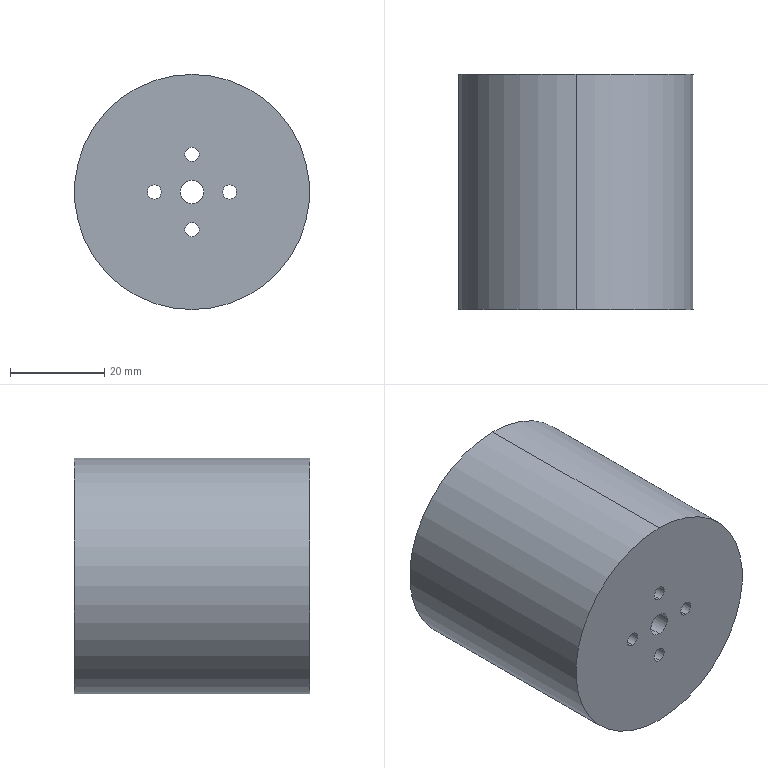Part | STEP file | Dial wheel | 1 solid | 19 faces | box 50 x 50 x 50 mm | volume 41621 mm3 | cylinder 14 | plane 3 | torus 2 | commonest cylinder face diameters 3 x8 5 x2 40 x2 50 x2
STEP:
#1=CARTESIAN_POINT('',(0.,0.,0.));
#2=DIRECTION('',(0.,0.,1.));
#3=DIRECTION('',(1.,0.,0.));
#4=AXIS2_PLACEMENT_3D('',#1,#2,#3);
#5=CARTESIAN_POINT('',(0.,5.,17.));
#6=VERTEX_POINT('',#5);
#7=CARTESIAN_POINT('',(0.,8.,20.));
#8=VERTEX_POINT('',#7);
#9=CARTESIAN_POINT('',(0.,8.,17.));
#10=DIRECTION('',(-1.,0.,0.));
#11=DIRECTION('',(0.,0.,1.));
#12=AXIS2_PLACEMENT_3D('',#9,#10,#11);
#13=CIRCLE('',#12,3.);
#14=CARTESIAN_POINT('',(0.,8.,0.));
#15=DIRECTION('',(0.,1.,0.));
#16=DIRECTION('',(0.,0.,1.));
#17=AXIS2_PLACEMENT_3D('',#14,#15,#16);
#18=TOROIDAL_SURFACE('',#17,17.,3.);
#19=CARTESIAN_POINT('',(6.283,0.));
#20=DIRECTION('',(0.,1.));
#21=VECTOR('',#20,1.);
#22=LINE('',#19,#21);
#23=(GEOMETRIC_REPRESENTATION_CONTEXT(2)PARAMETRIC_REPRESENTATION_CONTEXT()REPRESENTATION_CONTEXT('',''));
#24=DEFINITIONAL_REPRESENTATION('',(#22),#23);
#25=PCURVE('',#18,#24);
#26=CARTESIAN_POINT('',(0.,8.,0.));
#27=DIRECTION('',(0.,1.,0.));
#28=DIRECTION('',(0.,0.,1.));
#29=AXIS2_PLACEMENT_3D('',#26,#27,#28);
#30=TOROIDAL_SURFACE('',#29,17.,3.);
#31=CARTESIAN_POINT('',(0.,0.));
#32=DIRECTION('',(0.,1.));
#33=VECTOR('',#32,1.);
#34=LINE('',#31,#33);
#35=(GEOMETRIC_REPRESENTATION_CONTEXT(2)PARAMETRIC_REPRESENTATION_CONTEXT()REPRESENTATION_CONTEXT('',''));
#36=DEFINITIONAL_REPRESENTATION('',(#34),#35);
#37=PCURVE('',#30,#36);
#38=SURFACE_CURVE('',#13,(#25,#37),.PCURVE_S1.);
#39=EDGE_CURVE('',#6,#8,#38,.T.);
#40=ORIENTED_EDGE('',*,*,#39,.T.);
#41=CARTESIAN_POINT('',(0.,8.,-20.));
#42=VERTEX_POINT('',#41);
#43=CARTESIAN_POINT('',(0.,8.,0.));
#44=DIRECTION('',(0.,-1.,0.));
#45=DIRECTION('',(0.,0.,1.));
#46=AXIS2_PLACEMENT_3D('',#43,#44,#45);
#47=CIRCLE('',#46,20.);
#48=CARTESIAN_POINT('',(6.283,6.283));
#49=DIRECTION('',(-1.,0.));
#50=VECTOR('',#49,1.);
#51=LINE('',#48,#50);
#52=(GEOMETRIC_REPRESENTATION_CONTEXT(2)PARAMETRIC_REPRESENTATION_CONTEXT()REPRESENTATION_CONTEXT('',''));
#53=DEFINITIONAL_REPRESENTATION('',(#51),#52);
#54=PCURVE('',#18,#53);
#55=CARTESIAN_POINT('',(0.,5.,0.));
#56=DIRECTION('',(0.,1.,0.));
#57=DIRECTION('',(0.,0.,1.));
#58=AXIS2_PLACEMENT_3D('',#55,#56,#57);
#59=CYLINDRICAL_SURFACE('',#58,20.);
#60=CARTESIAN_POINT('',(6.283,3.));
#61=DIRECTION('',(-1.,0.));
#62=VECTOR('',#61,1.);
#63=LINE('',#60,#62);
#64=(GEOMETRIC_REPRESENTATION_CONTEXT(2)PARAMETRIC_REPRESENTATION_CONTEXT()REPRESENTATION_CONTEXT('',''));
#65=DEFINITIONAL_REPRESENTATION('',(#63),#64);
#66=PCURVE('',#59,#65);
#67=SURFACE_CURVE('',#47,(#54,#66),.PCURVE_S1.);
#68=EDGE_CURVE('',#8,#42,#67,.T.);
#69=ORIENTED_EDGE('',*,*,#68,.T.);
#70=CARTESIAN_POINT('',(0.,5.,-17.));
#71=VERTEX_POINT('',#70);
#72=CARTESIAN_POINT('',(0.,8.,-17.));
#73=DIRECTION('',(1.,0.,0.));
#74=DIRECTION('',(0.,0.,-1.));
#75=AXIS2_PLACEMENT_3D('',#72,#73,#74);
#76=CIRCLE('',#75,3.);
#77=CARTESIAN_POINT('',(3.142,0.));
#78=DIRECTION('',(0.,1.));
#79=VECTOR('',#78,1.);
#80=LINE('',#77,#79);
#81=(GEOMETRIC_REPRESENTATION_CONTEXT(2)PARAMETRIC_REPRESENTATION_CONTEXT()REPRESENTATION_CONTEXT('',''));
#82=DEFINITIONAL_REPRESENTATION('',(#80),#81);
#83=PCURVE('',#18,#82);
#84=CARTESIAN_POINT('',(3.142,0.));
#85=DIRECTION('',(0.,1.));
#86=VECTOR('',#85,1.);
#87=LINE('',#84,#86);
#88=(GEOMETRIC_REPRESENTATION_CONTEXT(2)PARAMETRIC_REPRESENTATION_CONTEXT()REPRESENTATION_CONTEXT('',''));
#89=DEFINITIONAL_REPRESENTATION('',(#87),#88);
#90=PCURVE('',#30,#89);
#91=SURFACE_CURVE('',#76,(#83,#90),.PCURVE_S1.);
#92=EDGE_CURVE('',#71,#42,#91,.T.);
#93=ORIENTED_EDGE('',*,*,#92,.F.);
#94=CARTESIAN_POINT('',(0.,5.,0.));
#95=DIRECTION('',(0.,1.,0.));
#96=DIRECTION('',(0.,0.,1.));
#97=AXIS2_PLACEMENT_3D('',#94,#95,#96);
#98=CIRCLE('',#97,17.);
#99=CARTESIAN_POINT('',(0.,4.712));
#100=DIRECTION('',(1.,0.));
#101=VECTOR('',#100,1.);
#102=LINE('',#99,#101);
#103=(GEOMETRIC_REPRESENTATION_CONTEXT(2)PARAMETRIC_REPRESENTATION_CONTEXT()REPRESENTATION_CONTEXT('',''));
#104=DEFINITIONAL_REPRESENTATION('',(#102),#103);
#105=PCURVE('',#18,#104);
#106=CARTESIAN_POINT('',(0.,5.,0.));
#107=DIRECTION('',(0.,1.,0.));
#108=DIRECTION('',(0.,0.,1.));
#109=AXIS2_PLACEMENT_3D('',#106,#107,#108);
#110=PLANE('',#109);
#111=CARTESIAN_POINT('',(0.,0.));
#112=DIRECTION('',(1.,0.));
#113=AXIS2_PLACEMENT_2D('',#111,#112);
#114=CIRCLE('',#113,17.);
#115=(GEOMETRIC_REPRESENTATION_CONTEXT(2)PARAMETRIC_REPRESENTATION_CONTEXT()REPRESENTATION_CONTEXT('',''));
#116=DEFINITIONAL_REPRESENTATION('',(#114),#115);
#117=PCURVE('',#110,#116);
#118=SURFACE_CURVE('',#98,(#105,#117),.PCURVE_S1.);
#119=EDGE_CURVE('',#71,#6,#118,.T.);
#120=ORIENTED_EDGE('',*,*,#119,.T.);
#121=EDGE_LOOP('',(#40,#69,#93,#120));
#122=FACE_BOUND('',#121,.F.);
#123=ADVANCED_FACE('',(#122),#18,.F.);
#124=CARTESIAN_POINT('',(0.,50.,20.));
#125=VERTEX_POINT('',#124);
#126=CARTESIAN_POINT('',(0.,5.,20.));
#127=DIRECTION('',(0.,1.,0.));
#128=VECTOR('',#127,1.);
#129=LINE('',#126,#128);
#130=CARTESIAN_POINT('',(6.283,0.));
#131=DIRECTION('',(0.,1.));
#132=VECTOR('',#131,1.);
#133=LINE('',#130,#132);
#134=(GEOMETRIC_REPRESENTATION_CONTEXT(2)PARAMETRIC_REPRESENTATION_CONTEXT()REPRESENTATION_CONTEXT('',''));
#135=DEFINITIONAL_REPRESENTATION('',(#133),#134);
#136=PCURVE('',#59,#135);
#137=CARTESIAN_POINT('',(0.,5.,0.));
#138=DIRECTION('',(0.,1.,0.));
#139=DIRECTION('',(0.,0.,1.));
#140=AXIS2_PLACEMENT_3D('',#137,#138,#139);
#141=CYLINDRICAL_SURFACE('',#140,20.);
#142=CARTESIAN_POINT('',(0.,0.));
#143=DIRECTION('',(0.,1.));
#144=VECTOR('',#143,1.);
#145=LINE('',#142,#144);
#146=(GEOMETRIC_REPRESENTATION_CONTEXT(2)PARAMETRIC_REPRESENTATION_CONTEXT()REPRESENTATION_CONTEXT('',''));
#147=DEFINITIONAL_REPRESENTATION('',(#145),#146);
#148=PCURVE('',#141,#147);
#149=SURFACE_CURVE('',#129,(#136,#148),.PCURVE_S1.);
#150=EDGE_CURVE('',#8,#125,#149,.T.);
#151=ORIENTED_EDGE('',*,*,#150,.T.);
#152=CARTESIAN_POINT('',(0.,50.,-20.));
#153=VERTEX_POINT('',#152);
#154=CARTESIAN_POINT('',(0.,50.,0.));
#155=DIRECTION('',(0.,1.,0.));
#156=DIRECTION('',(0.,0.,1.));
#157=AXIS2_PLACEMENT_3D('',#154,#155,#156);
#158=CIRCLE('',#157,20.);
#159=CARTESIAN_POINT('',(0.,45.));
#160=DIRECTION('',(1.,0.));
#161=VECTOR('',#160,1.);
#162=LINE('',#159,#161);
#163=(GEOMETRIC_REPRESENTATION_CONTEXT(2)PARAMETRIC_REPRESENTATION_CONTEXT()REPRESENTATION_CONTEXT('',''));
#164=DEFINITIONAL_REPRESENTATION('',(#162),#163);
#165=PCURVE('',#59,#164);
#166=CARTESIAN_POINT('',(0.,50.,0.));
#167=DIRECTION('',(0.,1.,0.));
#168=DIRECTION('',(0.,0.,1.));
#169=AXIS2_PLACEMENT_3D('',#166,#167,#168);
#170=PLANE('',#169);
#171=CARTESIAN_POINT('',(0.,0.));
#172=DIRECTION('',(1.,0.));
#173=AXIS2_PLACEMENT_2D('',#171,#172);
#174=CIRCLE('',#173,20.);
#175=(GEOMETRIC_REPRESENTATION_CONTEXT(2)PARAMETRIC_REPRESENTATION_CONTEXT()REPRESENTATION_CONTEXT('',''));
#176=DEFINITIONAL_REPRESENTATION('',(#174),#175);
#177=PCURVE('',#170,#176);
#178=SURFACE_CURVE('',#158,(#165,#177),.PCURVE_S1.);
#179=EDGE_CURVE('',#153,#125,#178,.T.);
#180=ORIENTED_EDGE('',*,*,#179,.F.);
#181=CARTESIAN_POINT('',(0.,5.,-20.));
#182=DIRECTION('',(0.,1.,0.));
#183=VECTOR('',#182,1.);
#184=LINE('',#181,#183);
#185=CARTESIAN_POINT('',(3.142,0.));
#186=DIRECTION('',(0.,1.));
#187=VECTOR('',#186,1.);
#188=LINE('',#185,#187);
#189=(GEOMETRIC_REPRESENTATION_CONTEXT(2)PARAMETRIC_REPRESENTATION_CONTEXT()REPRESENTATION_CONTEXT('',''));
#190=DEFINITIONAL_REPRESENTATION('',(#188),#189);
#191=PCURVE('',#59,#190);
#192=CARTESIAN_POINT('',(3.142,0.));
#193=DIRECTION('',(0.,1.));
#194=VECTOR('',#193,1.);
#195=LINE('',#192,#194);
#196=(GEOMETRIC_REPRESENTATION_CONTEXT(2)PARAMETRIC_REPRESENTATION_CONTEXT()REPRESENTATION_CONTEXT('',''));
#197=DEFINITIONAL_REPRESENTATION('',(#195),#196);
#198=PCURVE('',#141,#197);
#199=SURFACE_CURVE('',#184,(#191,#198),.PCURVE_S1.);
#200=EDGE_CURVE('',#42,#153,#199,.T.);
#201=ORIENTED_EDGE('',*,*,#200,.F.);
#202=ORIENTED_EDGE('',*,*,#68,.F.);
#203=EDGE_LOOP('',(#151,#180,#201,#202));
#204=FACE_BOUND('',#203,.F.);
#205=ADVANCED_FACE('',(#204),#59,.F.);
#206=CARTESIAN_POINT('',(0.,50.,25.));
#207=VERTEX_POINT('',#206);
#208=CARTESIAN_POINT('',(0.,50.,-25.));
#209=VERTEX_POINT('',#208);
#210=CARTESIAN_POINT('',(0.,50.,0.));
#211=DIRECTION('',(0.,1.,0.));
#212=DIRECTION('',(0.,0.,1.));
#213=AXIS2_PLACEMENT_3D('',#210,#211,#212);
#214=CIRCLE('',#213,25.);
#215=CARTESIAN_POINT('',(0.,50.,0.));
#216=DIRECTION('',(0.,-1.,0.));
#217=DIRECTION('',(0.,0.,-1.));
#218=AXIS2_PLACEMENT_3D('',#215,#216,#217);
#219=CYLINDRICAL_SURFACE('',#218,25.);
#220=CARTESIAN_POINT('',(3.142,0.));
#221=DIRECTION('',(-1.,0.));
#222=VECTOR('',#221,1.);
#223=LINE('',#220,#222);
#224=(GEOMETRIC_REPRESENTATION_CONTEXT(2)PARAMETRIC_REPRESENTATION_CONTEXT()REPRESENTATION_CONTEXT('',''));
#225=DEFINITIONAL_REPRESENTATION('',(#223),#224);
#226=PCURVE('',#219,#225);
#227=CARTESIAN_POINT('',(0.,0.));
#228=DIRECTION('',(1.,0.));
#229=AXIS2_PLACEMENT_2D('',#227,#228);
#230=CIRCLE('',#229,25.);
#231=(GEOMETRIC_REPRESENTATION_CONTEXT(2)PARAMETRIC_REPRESENTATION_CONTEXT()REPRESENTATION_CONTEXT('',''));
#232=DEFINITIONAL_REPRESENTATION('',(#230),#231);
#233=PCURVE('',#170,#232);
#234=SURFACE_CURVE('',#214,(#226,#233),.PCURVE_S1.);
#235=EDGE_CURVE('',#207,#209,#234,.T.);
#236=ORIENTED_EDGE('',*,*,#235,.F.);
#237=CARTESIAN_POINT('',(0.,0.,25.));
#238=VERTEX_POINT('',#237);
#239=CARTESIAN_POINT('',(0.,50.,25.));
#240=DIRECTION('',(0.,-1.,0.));
#241=VECTOR('',#240,1.);
#242=LINE('',#239,#241);
#243=CARTESIAN_POINT('',(3.142,0.));
#244=DIRECTION('',(0.,1.));
#245=VECTOR('',#244,1.);
#246=LINE('',#243,#245);
#247=(GEOMETRIC_REPRESENTATION_CONTEXT(2)PARAMETRIC_REPRESENTATION_CONTEXT()REPRESENTATION_CONTEXT('',''));
#248=DEFINITIONAL_REPRESENTATION('',(#246),#247);
#249=PCURVE('',#219,#248);
#250=CARTESIAN_POINT('',(0.,50.,0.));
#251=DIRECTION('',(0.,-1.,0.));
#252=DIRECTION('',(0.,0.,-1.));
#253=AXIS2_PLACEMENT_3D('',#250,#251,#252);
#254=CYLINDRICAL_SURFACE('',#253,25.);
#255=CARTESIAN_POINT('',(3.142,0.));
#256=DIRECTION('',(0.,1.));
#257=VECTOR('',#256,1.);
#258=LINE('',#255,#257);
#259=(GEOMETRIC_REPRESENTATION_CONTEXT(2)PARAMETRIC_REPRESENTATION_CONTEXT()REPRESENTATION_CONTEXT('',''));
#260=DEFINITIONAL_REPRESENTATION('',(#258),#259);
#261=PCURVE('',#254,#260);
#262=SURFACE_CURVE('',#242,(#249,#261),.PCURVE_S1.);
#263=EDGE_CURVE('',#207,#238,#262,.T.);
#264=ORIENTED_EDGE('',*,*,#263,.T.);
#265=CARTESIAN_POINT('',(0.,0.,-25.));
#266=VERTEX_POINT('',#265);
#267=CARTESIAN_POINT('',(0.,0.,0.));
#268=DIRECTION('',(0.,1.,0.));
#269=DIRECTION('',(0.,0.,1.));
#270=AXIS2_PLACEMENT_3D('',#267,#268,#269);
#271=CIRCLE('',#270,25.);
#272=CARTESIAN_POINT('',(3.142,50.));
#273=DIRECTION('',(-1.,0.));
#274=VECTOR('',#273,1.);
#275=LINE('',#272,#274);
#276=(GEOMETRIC_REPRESENTATION_CONTEXT(2)PARAMETRIC_REPRESENTATION_CONTEXT()REPRESENTATION_CONTEXT('',''));
#277=DEFINITIONAL_REPRESENTATION('',(#275),#276);
#278=PCURVE('',#219,#277);
#279=CARTESIAN_POINT('',(0.,0.,0.));
#280=DIRECTION('',(0.,1.,0.));
#281=DIRECTION('',(0.,0.,1.));
#282=AXIS2_PLACEMENT_3D('',#279,#280,#281);
#283=PLANE('',#282);
#284=CARTESIAN_POINT('',(0.,0.));
#285=DIRECTION('',(1.,0.));
#286=AXIS2_PLACEMENT_2D('',#284,#285);
#287=CIRCLE('',#286,25.);
#288=(GEOMETRIC_REPRESENTATION_CONTEXT(2)PARAMETRIC_REPRESENTATION_CONTEXT()REPRESENTATION_CONTEXT('',''));
#289=DEFINITIONAL_REPRESENTATION('',(#287),#288);
#290=PCURVE('',#283,#289);
#291=SURFACE_CURVE('',#271,(#278,#290),.PCURVE_S1.);
#292=EDGE_CURVE('',#238,#266,#291,.T.);
#293=ORIENTED_EDGE('',*,*,#292,.T.);
#294=CARTESIAN_POINT('',(0.,50.,-25.));
#295=DIRECTION('',(0.,-1.,0.));
#296=VECTOR('',#295,1.);
#297=LINE('',#294,#296);
#298=CARTESIAN_POINT('',(0.,0.));
#299=DIRECTION('',(0.,1.));
#300=VECTOR('',#299,1.);
#301=LINE('',#298,#300);
#302=(GEOMETRIC_REPRESENTATION_CONTEXT(2)PARAMETRIC_REPRESENTATION_CONTEXT()REPRESENTATION_CONTEXT('',''));
#303=DEFINITIONAL_REPRESENTATION('',(#301),#302);
#304=PCURVE('',#219,#303);
#305=CARTESIAN_POINT('',(6.283,0.));
#306=DIRECTION('',(0.,1.));
#307=VECTOR('',#306,1.);
#308=LINE('',#305,#307);
#309=(GEOMETRIC_REPRESENTATION_CONTEXT(2)PARAMETRIC_REPRESENTATION_CONTEXT()REPRESENTATION_CONTEXT('',''));
#310=DEFINITIONAL_REPRESENTATION('',(#308),#309);
#311=PCURVE('',#254,#310);
#312=SURFACE_CURVE('',#297,(#304,#311),.PCURVE_S1.);
#313=EDGE_CURVE('',#209,#266,#312,.T.);
#314=ORIENTED_EDGE('',*,*,#313,.F.);
#315=EDGE_LOOP('',(#236,#264,#293,#314));
#316=FACE_BOUND('',#315,.T.);
#317=ADVANCED_FACE('',(#316),#219,.T.);
#318=CARTESIAN_POINT('',(0.,5.,6.5));
#319=VERTEX_POINT('',#318);
#320=CARTESIAN_POINT('',(0.,0.,6.5));
#321=VERTEX_POINT('',#320);
#322=CARTESIAN_POINT('',(0.,128.,6.5));
#323=DIRECTION('',(0.,-1.,0.));
#324=VECTOR('',#323,1.);
#325=LINE('',#322,#324);
#326=CARTESIAN_POINT('',(0.,128.,8.));
#327=DIRECTION('',(0.,-1.,0.));
#328=DIRECTION('',(0.,0.,-1.));
#329=AXIS2_PLACEMENT_3D('',#326,#327,#328);
#330=CYLINDRICAL_SURFACE('',#329,1.5);
#331=CARTESIAN_POINT('',(6.283,0.));
#332=DIRECTION('',(0.,1.));
#333=VECTOR('',#332,1.);
#334=LINE('',#331,#333);
#335=(GEOMETRIC_REPRESENTATION_CONTEXT(2)PARAMETRIC_REPRESENTATION_CONTEXT()REPRESENTATION_CONTEXT('',''));
#336=DEFINITIONAL_REPRESENTATION('',(#334),#335);
#337=PCURVE('',#330,#336);
#338=CARTESIAN_POINT('',(0.,128.,8.));
#339=DIRECTION('',(0.,-1.,0.));
#340=DIRECTION('',(0.,0.,-1.));
#341=AXIS2_PLACEMENT_3D('',#338,#339,#340);
#342=CYLINDRICAL_SURFACE('',#341,1.5);
#343=CARTESIAN_POINT('',(0.,0.));
#344=DIRECTION('',(0.,1.));
#345=VECTOR('',#344,1.);
#346=LINE('',#343,#345);
#347=(GEOMETRIC_REPRESENTATION_CONTEXT(2)PARAMETRIC_REPRESENTATION_CONTEXT()REPRESENTATION_CONTEXT('',''));
#348=DEFINITIONAL_REPRESENTATION('',(#346),#347);
#349=PCURVE('',#342,#348);
#350=SURFACE_CURVE('',#325,(#337,#349),.PCURVE_S1.);
#351=EDGE_CURVE('',#319,#321,#350,.T.);
#352=ORIENTED_EDGE('',*,*,#351,.T.);
#353=CARTESIAN_POINT('',(0.,0.,9.5));
#354=VERTEX_POINT('',#353);
#355=CARTESIAN_POINT('',(0.,0.,8.));
#356=DIRECTION('',(0.,1.,0.));
#357=DIRECTION('',(0.,0.,1.));
#358=AXIS2_PLACEMENT_3D('',#355,#356,#357);
#359=CIRCLE('',#358,1.5);
#360=CARTESIAN_POINT('',(9.425,128.));
#361=DIRECTION('',(-1.,0.));
#362=VECTOR('',#361,1.);
#363=LINE('',#360,#362);
#364=(GEOMETRIC_REPRESENTATION_CONTEXT(2)PARAMETRIC_REPRESENTATION_CONTEXT()REPRESENTATION_CONTEXT('',''));
#365=DEFINITIONAL_REPRESENTATION('',(#363),#364);
#366=PCURVE('',#330,#365);
#367=CARTESIAN_POINT('',(8.,0.));
#368=DIRECTION('',(1.,0.));
#369=AXIS2_PLACEMENT_2D('',#367,#368);
#370=CIRCLE('',#369,1.5);
#371=(GEOMETRIC_REPRESENTATION_CONTEXT(2)PARAMETRIC_REPRESENTATION_CONTEXT()REPRESENTATION_CONTEXT('',''));
#372=DEFINITIONAL_REPRESENTATION('',(#370),#371);
#373=PCURVE('',#283,#372);
#374=SURFACE_CURVE('',#359,(#366,#373),.PCURVE_S1.);
#375=EDGE_CURVE('',#321,#354,#374,.T.);
#376=ORIENTED_EDGE('',*,*,#375,.T.);
#377=CARTESIAN_POINT('',(0.,5.,9.5));
#378=VERTEX_POINT('',#377);
#379=CARTESIAN_POINT('',(0.,128.,9.5));
#380=DIRECTION('',(0.,-1.,0.));
#381=VECTOR('',#380,1.);
#382=LINE('',#379,#381);
#383=CARTESIAN_POINT('',(3.142,0.));
#384=DIRECTION('',(0.,1.));
#385=VECTOR('',#384,1.);
#386=LINE('',#383,#385);
#387=(GEOMETRIC_REPRESENTATION_CONTEXT(2)PARAMETRIC_REPRESENTATION_CONTEXT()REPRESENTATION_CONTEXT('',''));
#388=DEFINITIONAL_REPRESENTATION('',(#386),#387);
#389=PCURVE('',#330,#388);
#390=CARTESIAN_POINT('',(3.142,0.));
#391=DIRECTION('',(0.,1.));
#392=VECTOR('',#391,1.);
#393=LINE('',#390,#392);
#394=(GEOMETRIC_REPRESENTATION_CONTEXT(2)PARAMETRIC_REPRESENTATION_CONTEXT()REPRESENTATION_CONTEXT('',''));
#395=DEFINITIONAL_REPRESENTATION('',(#393),#394);
#396=PCURVE('',#342,#395);
#397=SURFACE_CURVE('',#382,(#389,#396),.PCURVE_S1.);
#398=EDGE_CURVE('',#378,#354,#397,.T.);
#399=ORIENTED_EDGE('',*,*,#398,.F.);
#400=CARTESIAN_POINT('',(0.,5.,8.));
#401=DIRECTION('',(0.,-1.,0.));
#402=DIRECTION('',(0.,0.,1.));
#403=AXIS2_PLACEMENT_3D('',#400,#401,#402);
#404=CIRCLE('',#403,1.5);
#405=CARTESIAN_POINT('',(3.142,123.));
#406=DIRECTION('',(1.,0.));
#407=VECTOR('',#406,1.);
#408=LINE('',#405,#407);
#409=(GEOMETRIC_REPRESENTATION_CONTEXT(2)PARAMETRIC_REPRESENTATION_CONTEXT()REPRESENTATION_CONTEXT('',''));
#410=DEFINITIONAL_REPRESENTATION('',(#408),#409);
#411=PCURVE('',#330,#410);
#412=CARTESIAN_POINT('',(9.5,0.));
#413=CARTESIAN_POINT('',(9.5,-2.598));
#414=CARTESIAN_POINT('',(7.25,-1.299));
#415=CARTESIAN_POINT('',(5.,0.));
#416=CARTESIAN_POINT('',(7.25,1.299));
#417=CARTESIAN_POINT('',(9.5,2.598));
#418=CARTESIAN_POINT('',(9.5,0.));
#419=(BOUNDED_CURVE()B_SPLINE_CURVE(2,(#412,#413,#414,#415,#416,#417,#418),.UNSPECIFIED.,.T.,.F.)B_SPLINE_CURVE_WITH_KNOTS((1,2,2,2,2,1),(-2.094,0.,2.094,4.189,6.283,8.378),.UNSPECIFIED.)CURVE()GEOMETRIC_REPRESENTATION_ITEM()RATIONAL_B_SPLINE_CURVE((1.,0.5,1.,0.5,1.,0.5,1.))REPRESENTATION_ITEM(''));
#420=(GEOMETRIC_REPRESENTATION_CONTEXT(2)PARAMETRIC_REPRESENTATION_CONTEXT()REPRESENTATION_CONTEXT('',''));
#421=DEFINITIONAL_REPRESENTATION('',(#419),#420);
#422=PCURVE('',#110,#421);
#423=SURFACE_CURVE('',#404,(#411,#422),.PCURVE_S1.);
#424=EDGE_CURVE('',#378,#319,#423,.T.);
#425=ORIENTED_EDGE('',*,*,#424,.T.);
#426=EDGE_LOOP('',(#352,#376,#399,#425));
#427=FACE_BOUND('',#426,.F.);
#428=ADVANCED_FACE('',(#427),#330,.F.);
#429=CARTESIAN_POINT('',(0.,5.,-9.5));
#430=VERTEX_POINT('',#429);
#431=CARTESIAN_POINT('',(0.,0.,-9.5));
#432=VERTEX_POINT('',#431);
#433=CARTESIAN_POINT('',(0.,128.,-9.5));
#434=DIRECTION('',(0.,-1.,0.));
#435=VECTOR('',#434,1.);
#436=LINE('',#433,#435);
#437=CARTESIAN_POINT('',(0.,128.,-8.));
#438=DIRECTION('',(0.,-1.,0.));
#439=DIRECTION('',(0.,0.,-1.));
#440=AXIS2_PLACEMENT_3D('',#437,#438,#439);
#441=CYLINDRICAL_SURFACE('',#440,1.5);
#442=CARTESIAN_POINT('',(6.283,0.));
#443=DIRECTION('',(0.,1.));
#444=VECTOR('',#443,1.);
#445=LINE('',#442,#444);
#446=(GEOMETRIC_REPRESENTATION_CONTEXT(2)PARAMETRIC_REPRESENTATION_CONTEXT()REPRESENTATION_CONTEXT('',''));
#447=DEFINITIONAL_REPRESENTATION('',(#445),#446);
#448=PCURVE('',#441,#447);
#449=CARTESIAN_POINT('',(0.,128.,-8.));
#450=DIRECTION('',(0.,-1.,0.));
#451=DIRECTION('',(0.,0.,-1.));
#452=AXIS2_PLACEMENT_3D('',#449,#450,#451);
#453=CYLINDRICAL_SURFACE('',#452,1.5);
#454=CARTESIAN_POINT('',(0.,0.));
#455=DIRECTION('',(0.,1.));
#456=VECTOR('',#455,1.);
#457=LINE('',#454,#456);
#458=(GEOMETRIC_REPRESENTATION_CONTEXT(2)PARAMETRIC_REPRESENTATION_CONTEXT()REPRESENTATION_CONTEXT('',''));
#459=DEFINITIONAL_REPRESENTATION('',(#457),#458);
#460=PCURVE('',#453,#459);
#461=SURFACE_CURVE('',#436,(#448,#460),.PCURVE_S1.);
#462=EDGE_CURVE('',#430,#432,#461,.T.);
#463=ORIENTED_EDGE('',*,*,#462,.T.);
#464=CARTESIAN_POINT('',(0.,0.,-6.5));
#465=VERTEX_POINT('',#464);
#466=CARTESIAN_POINT('',(0.,0.,-8.));
#467=DIRECTION('',(0.,1.,0.));
#468=DIRECTION('',(0.,0.,1.));
#469=AXIS2_PLACEMENT_3D('',#466,#467,#468);
#470=CIRCLE('',#469,1.5);
#471=CARTESIAN_POINT('',(9.425,128.));
#472=DIRECTION('',(-1.,0.));
#473=VECTOR('',#472,1.);
#474=LINE('',#471,#473);
#475=(GEOMETRIC_REPRESENTATION_CONTEXT(2)PARAMETRIC_REPRESENTATION_CONTEXT()REPRESENTATION_CONTEXT('',''));
#476=DEFINITIONAL_REPRESENTATION('',(#474),#475);
#477=PCURVE('',#441,#476);
#478=CARTESIAN_POINT('',(-8.,0.));
#479=DIRECTION('',(1.,0.));
#480=AXIS2_PLACEMENT_2D('',#478,#479);
#481=CIRCLE('',#480,1.5);
#482=(GEOMETRIC_REPRESENTATION_CONTEXT(2)PARAMETRIC_REPRESENTATION_CONTEXT()REPRESENTATION_CONTEXT('',''));
#483=DEFINITIONAL_REPRESENTATION('',(#481),#482);
#484=PCURVE('',#283,#483);
#485=SURFACE_CURVE('',#470,(#477,#484),.PCURVE_S1.);
#486=EDGE_CURVE('',#432,#465,#485,.T.);
#487=ORIENTED_EDGE('',*,*,#486,.T.);
#488=CARTESIAN_POINT('',(0.,5.,-6.5));
#489=VERTEX_POINT('',#488);
#490=CARTESIAN_POINT('',(0.,128.,-6.5));
#491=DIRECTION('',(0.,-1.,0.));
#492=VECTOR('',#491,1.);
#493=LINE('',#490,#492);
#494=CARTESIAN_POINT('',(3.142,0.));
#495=DIRECTION('',(0.,1.));
#496=VECTOR('',#495,1.);
#497=LINE('',#494,#496);
#498=(GEOMETRIC_REPRESENTATION_CONTEXT(2)PARAMETRIC_REPRESENTATION_CONTEXT()REPRESENTATION_CONTEXT('',''));
#499=DEFINITIONAL_REPRESENTATION('',(#497),#498);
#500=PCURVE('',#441,#499);
#501=CARTESIAN_POINT('',(3.142,0.));
#502=DIRECTION('',(0.,1.));
#503=VECTOR('',#502,1.);
#504=LINE('',#501,#503);
#505=(GEOMETRIC_REPRESENTATION_CONTEXT(2)PARAMETRIC_REPRESENTATION_CONTEXT()REPRESENTATION_CONTEXT('',''));
#506=DEFINITIONAL_REPRESENTATION('',(#504),#505);
#507=PCURVE('',#453,#506);
#508=SURFACE_CURVE('',#493,(#500,#507),.PCURVE_S1.);
#509=EDGE_CURVE('',#489,#465,#508,.T.);
#510=ORIENTED_EDGE('',*,*,#509,.F.);
#511=CARTESIAN_POINT('',(0.,5.,-8.));
#512=DIRECTION('',(0.,-1.,0.));
#513=DIRECTION('',(0.,0.,1.));
#514=AXIS2_PLACEMENT_3D('',#511,#512,#513);
#515=CIRCLE('',#514,1.5);
#516=CARTESIAN_POINT('',(3.142,123.));
#517=DIRECTION('',(1.,0.));
#518=VECTOR('',#517,1.);
#519=LINE('',#516,#518);
#520=(GEOMETRIC_REPRESENTATION_CONTEXT(2)PARAMETRIC_REPRESENTATION_CONTEXT()REPRESENTATION_CONTEXT('',''));
#521=DEFINITIONAL_REPRESENTATION('',(#519),#520);
#522=PCURVE('',#441,#521);
#523=CARTESIAN_POINT('',(-6.5,0.));
#524=CARTESIAN_POINT('',(-6.5,-2.598));
#525=CARTESIAN_POINT('',(-8.75,-1.299));
#526=CARTESIAN_POINT('',(-11.,0.));
#527=CARTESIAN_POINT('',(-8.75,1.299));
#528=CARTESIAN_POINT('',(-6.5,2.598));
#529=CARTESIAN_POINT('',(-6.5,0.));
#530=(BOUNDED_CURVE()B_SPLINE_CURVE(2,(#523,#524,#525,#526,#527,#528,#529),.UNSPECIFIED.,.T.,.F.)B_SPLINE_CURVE_WITH_KNOTS((1,2,2,2,2,1),(-2.094,0.,2.094,4.189,6.283,8.378),.UNSPECIFIED.)CURVE()GEOMETRIC_REPRESENTATION_ITEM()RATIONAL_B_SPLINE_CURVE((1.,0.5,1.,0.5,1.,0.5,1.))REPRESENTATION_ITEM(''));
#531=(GEOMETRIC_REPRESENTATION_CONTEXT(2)PARAMETRIC_REPRESENTATION_CONTEXT()REPRESENTATION_CONTEXT('',''));
#532=DEFINITIONAL_REPRESENTATION('',(#530),#531);
#533=PCURVE('',#110,#532);
#534=SURFACE_CURVE('',#515,(#522,#533),.PCURVE_S1.);
#535=EDGE_CURVE('',#489,#430,#534,.T.);
#536=ORIENTED_EDGE('',*,*,#535,.T.);
#537=EDGE_LOOP('',(#463,#487,#510,#536));
#538=FACE_BOUND('',#537,.F.);
#539=ADVANCED_FACE('',(#538),#441,.F.);
#540=CARTESIAN_POINT('',(-8.,5.,-1.5));
#541=VERTEX_POINT('',#540);
#542=CARTESIAN_POINT('',(-8.,0.,-1.5));
#543=VERTEX_POINT('',#542);
#544=CARTESIAN_POINT('',(-8.,128.,-1.5));
#545=DIRECTION('',(0.,-1.,0.));
#546=VECTOR('',#545,1.);
#547=LINE('',#544,#546);
#548=CARTESIAN_POINT('',(-8.,128.,0.));
#549=DIRECTION('',(0.,-1.,0.));
#550=DIRECTION('',(0.,0.,-1.));
#551=AXIS2_PLACEMENT_3D('',#548,#549,#550);
#552=CYLINDRICAL_SURFACE('',#551,1.5);
#553=CARTESIAN_POINT('',(6.283,0.));
#554=DIRECTION('',(0.,1.));
#555=VECTOR('',#554,1.);
#556=LINE('',#553,#555);
#557=(GEOMETRIC_REPRESENTATION_CONTEXT(2)PARAMETRIC_REPRESENTATION_CONTEXT()REPRESENTATION_CONTEXT('',''));
#558=DEFINITIONAL_REPRESENTATION('',(#556),#557);
#559=PCURVE('',#552,#558);
#560=CARTESIAN_POINT('',(-8.,128.,0.));
#561=DIRECTION('',(0.,-1.,0.));
#562=DIRECTION('',(0.,0.,-1.));
#563=AXIS2_PLACEMENT_3D('',#560,#561,#562);
#564=CYLINDRICAL_SURFACE('',#563,1.5);
#565=CARTESIAN_POINT('',(0.,0.));
#566=DIRECTION('',(0.,1.));
#567=VECTOR('',#566,1.);
#568=LINE('',#565,#567);
#569=(GEOMETRIC_REPRESENTATION_CONTEXT(2)PARAMETRIC_REPRESENTATION_CONTEXT()REPRESENTATION_CONTEXT('',''));
#570=DEFINITIONAL_REPRESENTATION('',(#568),#569);
#571=PCURVE('',#564,#570);
#572=SURFACE_CURVE('',#547,(#559,#571),.PCURVE_S1.);
#573=EDGE_CURVE('',#541,#543,#572,.T.);
#574=ORIENTED_EDGE('',*,*,#573,.T.);
#575=CARTESIAN_POINT('',(-8.,0.,1.5));
#576=VERTEX_POINT('',#575);
#577=CARTESIAN_POINT('',(-8.,0.,0.));
#578=DIRECTION('',(0.,1.,0.));
#579=DIRECTION('',(0.,0.,1.));
#580=AXIS2_PLACEMENT_3D('',#577,#578,#579);
#581=CIRCLE('',#580,1.5);
#582=CARTESIAN_POINT('',(9.425,128.));
#583=DIRECTION('',(-1.,0.));
#584=VECTOR('',#583,1.);
#585=LINE('',#582,#584);
#586=(GEOMETRIC_REPRESENTATION_CONTEXT(2)PARAMETRIC_REPRESENTATION_CONTEXT()REPRESENTATION_CONTEXT('',''));
#587=DEFINITIONAL_REPRESENTATION('',(#585),#586);
#588=PCURVE('',#552,#587);
#589=CARTESIAN_POINT('',(0.,-8.));
#590=DIRECTION('',(1.,0.));
#591=AXIS2_PLACEMENT_2D('',#589,#590);
#592=CIRCLE('',#591,1.5);
#593=(GEOMETRIC_REPRESENTATION_CONTEXT(2)PARAMETRIC_REPRESENTATION_CONTEXT()REPRESENTATION_CONTEXT('',''));
#594=DEFINITIONAL_REPRESENTATION('',(#592),#593);
#595=PCURVE('',#283,#594);
#596=SURFACE_CURVE('',#581,(#588,#595),.PCURVE_S1.);
#597=EDGE_CURVE('',#543,#576,#596,.T.);
#598=ORIENTED_EDGE('',*,*,#597,.T.);
#599=CARTESIAN_POINT('',(-8.,5.,1.5));
#600=VERTEX_POINT('',#599);
#601=CARTESIAN_POINT('',(-8.,128.,1.5));
#602=DIRECTION('',(0.,-1.,0.));
#603=VECTOR('',#602,1.);
#604=LINE('',#601,#603);
#605=CARTESIAN_POINT('',(3.142,0.));
#606=DIRECTION('',(0.,1.));
#607=VECTOR('',#606,1.);
#608=LINE('',#605,#607);
#609=(GEOMETRIC_REPRESENTATION_CONTEXT(2)PARAMETRIC_REPRESENTATION_CONTEXT()REPRESENTATION_CONTEXT('',''));
#610=DEFINITIONAL_REPRESENTATION('',(#608),#609);
#611=PCURVE('',#552,#610);
#612=CARTESIAN_POINT('',(3.142,0.));
#613=DIRECTION('',(0.,1.));
#614=VECTOR('',#613,1.);
#615=LINE('',#612,#614);
#616=(GEOMETRIC_REPRESENTATION_CONTEXT(2)PARAMETRIC_REPRESENTATION_CONTEXT()REPRESENTATION_CONTEXT('',''));
#617=DEFINITIONAL_REPRESENTATION('',(#615),#616);
#618=PCURVE('',#564,#617);
#619=SURFACE_CURVE('',#604,(#611,#618),.PCURVE_S1.);
#620=EDGE_CURVE('',#600,#576,#619,.T.);
#621=ORIENTED_EDGE('',*,*,#620,.F.);
#622=CARTESIAN_POINT('',(-8.,5.,0.));
#623=DIRECTION('',(0.,-1.,0.));
#624=DIRECTION('',(0.,0.,1.));
#625=AXIS2_PLACEMENT_3D('',#622,#623,#624);
#626=CIRCLE('',#625,1.5);
#627=CARTESIAN_POINT('',(3.142,123.));
#628=DIRECTION('',(1.,0.));
#629=VECTOR('',#628,1.);
#630=LINE('',#627,#629);
#631=(GEOMETRIC_REPRESENTATION_CONTEXT(2)PARAMETRIC_REPRESENTATION_CONTEXT()REPRESENTATION_CONTEXT('',''));
#632=DEFINITIONAL_REPRESENTATION('',(#630),#631);
#633=PCURVE('',#552,#632);
#634=CARTESIAN_POINT('',(1.5,-8.));
#635=CARTESIAN_POINT('',(1.5,-10.598));
#636=CARTESIAN_POINT('',(-0.75,-9.299));
#637=CARTESIAN_POINT('',(-3.,-8.));
#638=CARTESIAN_POINT('',(-0.75,-6.701));
#639=CARTESIAN_POINT('',(1.5,-5.402));
#640=CARTESIAN_POINT('',(1.5,-8.));
#641=(BOUNDED_CURVE()B_SPLINE_CURVE(2,(#634,#635,#636,#637,#638,#639,#640),.UNSPECIFIED.,.T.,.F.)B_SPLINE_CURVE_WITH_KNOTS((1,2,2,2,2,1),(-2.094,0.,2.094,4.189,6.283,8.378),.UNSPECIFIED.)CURVE()GEOMETRIC_REPRESENTATION_ITEM()RATIONAL_B_SPLINE_CURVE((1.,0.5,1.,0.5,1.,0.5,1.))REPRESENTATION_ITEM(''));
#642=(GEOMETRIC_REPRESENTATION_CONTEXT(2)PARAMETRIC_REPRESENTATION_CONTEXT()REPRESENTATION_CONTEXT('',''));
#643=DEFINITIONAL_REPRESENTATION('',(#641),#642);
#644=PCURVE('',#110,#643);
#645=SURFACE_CURVE('',#626,(#633,#644),.PCURVE_S1.);
#646=EDGE_CURVE('',#600,#541,#645,.T.);
#647=ORIENTED_EDGE('',*,*,#646,.T.);
#648=EDGE_LOOP('',(#574,#598,#621,#647));
#649=FACE_BOUND('',#648,.F.);
#650=ADVANCED_FACE('',(#649),#552,.F.);
#651=CARTESIAN_POINT('',(8.,5.,-1.5));
#652=VERTEX_POINT('',#651);
#653=CARTESIAN_POINT('',(8.,0.,-1.5));
#654=VERTEX_POINT('',#653);
#655=CARTESIAN_POINT('',(8.,128.,-1.5));
#656=DIRECTION('',(0.,-1.,0.));
#657=VECTOR('',#656,1.);
#658=LINE('',#655,#657);
#659=CARTESIAN_POINT('',(8.,128.,0.));
#660=DIRECTION('',(0.,-1.,0.));
#661=DIRECTION('',(0.,0.,-1.));
#662=AXIS2_PLACEMENT_3D('',#659,#660,#661);
#663=CYLINDRICAL_SURFACE('',#662,1.5);
#664=CARTESIAN_POINT('',(6.283,0.));
#665=DIRECTION('',(0.,1.));
#666=VECTOR('',#665,1.);
#667=LINE('',#664,#666);
#668=(GEOMETRIC_REPRESENTATION_CONTEXT(2)PARAMETRIC_REPRESENTATION_CONTEXT()REPRESENTATION_CONTEXT('',''));
#669=DEFINITIONAL_REPRESENTATION('',(#667),#668);
#670=PCURVE('',#663,#669);
#671=CARTESIAN_POINT('',(8.,128.,0.));
#672=DIRECTION('',(0.,-1.,0.));
#673=DIRECTION('',(0.,0.,-1.));
#674=AXIS2_PLACEMENT_3D('',#671,#672,#673);
#675=CYLINDRICAL_SURFACE('',#674,1.5);
#676=CARTESIAN_POINT('',(0.,0.));
#677=DIRECTION('',(0.,1.));
#678=VECTOR('',#677,1.);
#679=LINE('',#676,#678);
#680=(GEOMETRIC_REPRESENTATION_CONTEXT(2)PARAMETRIC_REPRESENTATION_CONTEXT()REPRESENTATION_CONTEXT('',''));
#681=DEFINITIONAL_REPRESENTATION('',(#679),#680);
#682=PCURVE('',#675,#681);
#683=SURFACE_CURVE('',#658,(#670,#682),.PCURVE_S1.);
#684=EDGE_CURVE('',#652,#654,#683,.T.);
#685=ORIENTED_EDGE('',*,*,#684,.T.);
#686=CARTESIAN_POINT('',(8.,0.,1.5));
#687=VERTEX_POINT('',#686);
#688=CARTESIAN_POINT('',(8.,0.,0.));
#689=DIRECTION('',(0.,1.,0.));
#690=DIRECTION('',(0.,0.,1.));
#691=AXIS2_PLACEMENT_3D('',#688,#689,#690);
#692=CIRCLE('',#691,1.5);
#693=CARTESIAN_POINT('',(9.425,128.));
#694=DIRECTION('',(-1.,0.));
#695=VECTOR('',#694,1.);
#696=LINE('',#693,#695);
#697=(GEOMETRIC_REPRESENTATION_CONTEXT(2)PARAMETRIC_REPRESENTATION_CONTEXT()REPRESENTATION_CONTEXT('',''));
#698=DEFINITIONAL_REPRESENTATION('',(#696),#697);
#699=PCURVE('',#663,#698);
#700=CARTESIAN_POINT('',(0.,8.));
#701=DIRECTION('',(1.,0.));
#702=AXIS2_PLACEMENT_2D('',#700,#701);
#703=CIRCLE('',#702,1.5);
#704=(GEOMETRIC_REPRESENTATION_CONTEXT(2)PARAMETRIC_REPRESENTATION_CONTEXT()REPRESENTATION_CONTEXT('',''));
#705=DEFINITIONAL_REPRESENTATION('',(#703),#704);
#706=PCURVE('',#283,#705);
#707=SURFACE_CURVE('',#692,(#699,#706),.PCURVE_S1.);
#708=EDGE_CURVE('',#654,#687,#707,.T.);
#709=ORIENTED_EDGE('',*,*,#708,.T.);
#710=CARTESIAN_POINT('',(8.,5.,1.5));
#711=VERTEX_POINT('',#710);
#712=CARTESIAN_POINT('',(8.,128.,1.5));
#713=DIRECTION('',(0.,-1.,0.));
#714=VECTOR('',#713,1.);
#715=LINE('',#712,#714);
#716=CARTESIAN_POINT('',(3.142,0.));
#717=DIRECTION('',(0.,1.));
#718=VECTOR('',#717,1.);
#719=LINE('',#716,#718);
#720=(GEOMETRIC_REPRESENTATION_CONTEXT(2)PARAMETRIC_REPRESENTATION_CONTEXT()REPRESENTATION_CONTEXT('',''));
#721=DEFINITIONAL_REPRESENTATION('',(#719),#720);
#722=PCURVE('',#663,#721);
#723=CARTESIAN_POINT('',(3.142,0.));
#724=DIRECTION('',(0.,1.));
#725=VECTOR('',#724,1.);
#726=LINE('',#723,#725);
#727=(GEOMETRIC_REPRESENTATION_CONTEXT(2)PARAMETRIC_REPRESENTATION_CONTEXT()REPRESENTATION_CONTEXT('',''));
#728=DEFINITIONAL_REPRESENTATION('',(#726),#727);
#729=PCURVE('',#675,#728);
#730=SURFACE_CURVE('',#715,(#722,#729),.PCURVE_S1.);
#731=EDGE_CURVE('',#711,#687,#730,.T.);
#732=ORIENTED_EDGE('',*,*,#731,.F.);
#733=CARTESIAN_POINT('',(8.,5.,0.));
#734=DIRECTION('',(0.,-1.,0.));
#735=DIRECTION('',(0.,0.,1.));
#736=AXIS2_PLACEMENT_3D('',#733,#734,#735);
#737=CIRCLE('',#736,1.5);
#738=CARTESIAN_POINT('',(3.142,123.));
#739=DIRECTION('',(1.,0.));
#740=VECTOR('',#739,1.);
#741=LINE('',#738,#740);
#742=(GEOMETRIC_REPRESENTATION_CONTEXT(2)PARAMETRIC_REPRESENTATION_CONTEXT()REPRESENTATION_CONTEXT('',''));
#743=DEFINITIONAL_REPRESENTATION('',(#741),#742);
#744=PCURVE('',#663,#743);
#745=CARTESIAN_POINT('',(1.5,8.));
#746=CARTESIAN_POINT('',(1.5,5.402));
#747=CARTESIAN_POINT('',(-0.75,6.701));
#748=CARTESIAN_POINT('',(-3.,8.));
#749=CARTESIAN_POINT('',(-0.75,9.299));
#750=CARTESIAN_POINT('',(1.5,10.598));
#751=CARTESIAN_POINT('',(1.5,8.));
#752=(BOUNDED_CURVE()B_SPLINE_CURVE(2,(#745,#746,#747,#748,#749,#750,#751),.UNSPECIFIED.,.T.,.F.)B_SPLINE_CURVE_WITH_KNOTS((1,2,2,2,2,1),(-2.094,0.,2.094,4.189,6.283,8.378),.UNSPECIFIED.)CURVE()GEOMETRIC_REPRESENTATION_ITEM()RATIONAL_B_SPLINE_CURVE((1.,0.5,1.,0.5,1.,0.5,1.))REPRESENTATION_ITEM(''));
#753=(GEOMETRIC_REPRESENTATION_CONTEXT(2)PARAMETRIC_REPRESENTATION_CONTEXT()REPRESENTATION_CONTEXT('',''));
#754=DEFINITIONAL_REPRESENTATION('',(#752),#753);
#755=PCURVE('',#110,#754);
#756=SURFACE_CURVE('',#737,(#744,#755),.PCURVE_S1.);
#757=EDGE_CURVE('',#711,#652,#756,.T.);
#758=ORIENTED_EDGE('',*,*,#757,.T.);
#759=EDGE_LOOP('',(#685,#709,#732,#758));
#760=FACE_BOUND('',#759,.F.);
#761=ADVANCED_FACE('',(#760),#663,.F.);
#762=CARTESIAN_POINT('',(0.,5.,-2.5));
#763=VERTEX_POINT('',#762);
#764=CARTESIAN_POINT('',(0.,0.,-2.5));
#765=VERTEX_POINT('',#764);
#766=CARTESIAN_POINT('',(0.,50.,-2.5));
#767=DIRECTION('',(0.,-1.,0.));
#768=VECTOR('',#767,1.);
#769=LINE('',#766,#768);
#770=CARTESIAN_POINT('',(0.,50.,0.));
#771=DIRECTION('',(0.,-1.,0.));
#772=DIRECTION('',(0.,0.,-1.));
#773=AXIS2_PLACEMENT_3D('',#770,#771,#772);
#774=CYLINDRICAL_SURFACE('',#773,2.5);
#775=CARTESIAN_POINT('',(6.283,0.));
#776=DIRECTION('',(0.,1.));
#777=VECTOR('',#776,1.);
#778=LINE('',#775,#777);
#779=(GEOMETRIC_REPRESENTATION_CONTEXT(2)PARAMETRIC_REPRESENTATION_CONTEXT()REPRESENTATION_CONTEXT('',''));
#780=DEFINITIONAL_REPRESENTATION('',(#778),#779);
#781=PCURVE('',#774,#780);
#782=CARTESIAN_POINT('',(0.,50.,0.));
#783=DIRECTION('',(0.,-1.,0.));
#784=DIRECTION('',(0.,0.,-1.));
#785=AXIS2_PLACEMENT_3D('',#782,#783,#784);
#786=CYLINDRICAL_SURFACE('',#785,2.5);
#787=CARTESIAN_POINT('',(0.,0.));
#788=DIRECTION('',(0.,1.));
#789=VECTOR('',#788,1.);
#790=LINE('',#787,#789);
#791=(GEOMETRIC_REPRESENTATION_CONTEXT(2)PARAMETRIC_REPRESENTATION_CONTEXT()REPRESENTATION_CONTEXT('',''));
#792=DEFINITIONAL_REPRESENTATION('',(#790),#791);
#793=PCURVE('',#786,#792);
#794=SURFACE_CURVE('',#769,(#781,#793),.PCURVE_S1.);
#795=EDGE_CURVE('',#763,#765,#794,.T.);
#796=ORIENTED_EDGE('',*,*,#795,.T.);
#797=CARTESIAN_POINT('',(0.,0.,2.5));
#798=VERTEX_POINT('',#797);
#799=CARTESIAN_POINT('',(0.,0.,0.));
#800=DIRECTION('',(0.,1.,0.));
#801=DIRECTION('',(0.,0.,1.));
#802=AXIS2_PLACEMENT_3D('',#799,#800,#801);
#803=CIRCLE('',#802,2.5);
#804=CARTESIAN_POINT('',(9.425,50.));
#805=DIRECTION('',(-1.,0.));
#806=VECTOR('',#805,1.);
#807=LINE('',#804,#806);
#808=(GEOMETRIC_REPRESENTATION_CONTEXT(2)PARAMETRIC_REPRESENTATION_CONTEXT()REPRESENTATION_CONTEXT('',''));
#809=DEFINITIONAL_REPRESENTATION('',(#807),#808);
#810=PCURVE('',#774,#809);
#811=CARTESIAN_POINT('',(0.,0.));
#812=DIRECTION('',(1.,0.));
#813=AXIS2_PLACEMENT_2D('',#811,#812);
#814=CIRCLE('',#813,2.5);
#815=(GEOMETRIC_REPRESENTATION_CONTEXT(2)PARAMETRIC_REPRESENTATION_CONTEXT()REPRESENTATION_CONTEXT('',''));
#816=DEFINITIONAL_REPRESENTATION('',(#814),#815);
#817=PCURVE('',#283,#816);
#818=SURFACE_CURVE('',#803,(#810,#817),.PCURVE_S1.);
#819=EDGE_CURVE('',#765,#798,#818,.T.);
#820=ORIENTED_EDGE('',*,*,#819,.T.);
#821=CARTESIAN_POINT('',(0.,5.,2.5));
#822=VERTEX_POINT('',#821);
#823=CARTESIAN_POINT('',(0.,50.,2.5));
#824=DIRECTION('',(0.,-1.,0.));
#825=VECTOR('',#824,1.);
#826=LINE('',#823,#825);
#827=CARTESIAN_POINT('',(3.142,0.));
#828=DIRECTION('',(0.,1.));
#829=VECTOR('',#828,1.);
#830=LINE('',#827,#829);
#831=(GEOMETRIC_REPRESENTATION_CONTEXT(2)PARAMETRIC_REPRESENTATION_CONTEXT()REPRESENTATION_CONTEXT('',''));
#832=DEFINITIONAL_REPRESENTATION('',(#830),#831);
#833=PCURVE('',#774,#832);
#834=CARTESIAN_POINT('',(3.142,0.));
#835=DIRECTION('',(0.,1.));
#836=VECTOR('',#835,1.);
#837=LINE('',#834,#836);
#838=(GEOMETRIC_REPRESENTATION_CONTEXT(2)PARAMETRIC_REPRESENTATION_CONTEXT()REPRESENTATION_CONTEXT('',''));
#839=DEFINITIONAL_REPRESENTATION('',(#837),#838);
#840=PCURVE('',#786,#839);
#841=SURFACE_CURVE('',#826,(#833,#840),.PCURVE_S1.);
#842=EDGE_CURVE('',#822,#798,#841,.T.);
#843=ORIENTED_EDGE('',*,*,#842,.F.);
#844=CARTESIAN_POINT('',(0.,5.,0.));
#845=DIRECTION('',(0.,1.,0.));
#846=DIRECTION('',(0.,0.,1.));
#847=AXIS2_PLACEMENT_3D('',#844,#845,#846);
#848=CIRCLE('',#847,2.5);
#849=CARTESIAN_POINT('',(9.425,45.));
#850=DIRECTION('',(-1.,0.));
#851=VECTOR('',#850,1.);
#852=LINE('',#849,#851);
#853=(GEOMETRIC_REPRESENTATION_CONTEXT(2)PARAMETRIC_REPRESENTATION_CONTEXT()REPRESENTATION_CONTEXT('',''));
#854=DEFINITIONAL_REPRESENTATION('',(#852),#853);
#855=PCURVE('',#774,#854);
#856=CARTESIAN_POINT('',(0.,0.));
#857=DIRECTION('',(1.,0.));
#858=AXIS2_PLACEMENT_2D('',#856,#857);
#859=CIRCLE('',#858,2.5);
#860=(GEOMETRIC_REPRESENTATION_CONTEXT(2)PARAMETRIC_REPRESENTATION_CONTEXT()REPRESENTATION_CONTEXT('',''));
#861=DEFINITIONAL_REPRESENTATION('',(#859),#860);
#862=PCURVE('',#110,#861);
#863=SURFACE_CURVE('',#848,(#855,#862),.PCURVE_S1.);
#864=EDGE_CURVE('',#763,#822,#863,.T.);
#865=ORIENTED_EDGE('',*,*,#864,.F.);
#866=EDGE_LOOP('',(#796,#820,#843,#865));
#867=FACE_BOUND('',#866,.F.);
#868=ADVANCED_FACE('',(#867),#774,.F.);
#869=CARTESIAN_POINT('',(0.,0.,0.));
#870=DIRECTION('',(0.,1.,0.));
#871=DIRECTION('',(0.,0.,1.));
#872=AXIS2_PLACEMENT_3D('',#869,#870,#871);
#873=CIRCLE('',#872,2.5);
#874=CARTESIAN_POINT('',(3.142,50.));
#875=DIRECTION('',(-1.,0.));
#876=VECTOR('',#875,1.);
#877=LINE('',#874,#876);
#878=(GEOMETRIC_REPRESENTATION_CONTEXT(2)PARAMETRIC_REPRESENTATION_CONTEXT()REPRESENTATION_CONTEXT('',''));
#879=DEFINITIONAL_REPRESENTATION('',(#877),#878);
#880=PCURVE('',#786,#879);
#881=CARTESIAN_POINT('',(0.,0.));
#882=DIRECTION('',(1.,0.));
#883=AXIS2_PLACEMENT_2D('',#881,#882);
#884=CIRCLE('',#883,2.5);
#885=(GEOMETRIC_REPRESENTATION_CONTEXT(2)PARAMETRIC_REPRESENTATION_CONTEXT()REPRESENTATION_CONTEXT('',''));
#886=DEFINITIONAL_REPRESENTATION('',(#884),#885);
#887=PCURVE('',#283,#886);
#888=SURFACE_CURVE('',#873,(#880,#887),.PCURVE_S1.);
#889=EDGE_CURVE('',#798,#765,#888,.T.);
#890=ORIENTED_EDGE('',*,*,#889,.T.);
#891=ORIENTED_EDGE('',*,*,#795,.F.);
#892=CARTESIAN_POINT('',(0.,5.,0.));
#893=DIRECTION('',(0.,1.,0.));
#894=DIRECTION('',(0.,0.,1.));
#895=AXIS2_PLACEMENT_3D('',#892,#893,#894);
#896=CIRCLE('',#895,2.5);
#897=CARTESIAN_POINT('',(3.142,45.));
#898=DIRECTION('',(-1.,0.));
#899=VECTOR('',#898,1.);
#900=LINE('',#897,#899);
#901=(GEOMETRIC_REPRESENTATION_CONTEXT(2)PARAMETRIC_REPRESENTATION_CONTEXT()REPRESENTATION_CONTEXT('',''));
#902=DEFINITIONAL_REPRESENTATION('',(#900),#901);
#903=PCURVE('',#786,#902);
#904=CARTESIAN_POINT('',(0.,0.));
#905=DIRECTION('',(1.,0.));
#906=AXIS2_PLACEMENT_2D('',#904,#905);
#907=CIRCLE('',#906,2.5);
#908=(GEOMETRIC_REPRESENTATION_CONTEXT(2)PARAMETRIC_REPRESENTATION_CONTEXT()REPRESENTATION_CONTEXT('',''));
#909=DEFINITIONAL_REPRESENTATION('',(#907),#908);
#910=PCURVE('',#110,#909);
#911=SURFACE_CURVE('',#896,(#903,#910),.PCURVE_S1.);
#912=EDGE_CURVE('',#822,#763,#911,.T.);
#913=ORIENTED_EDGE('',*,*,#912,.F.);
#914=ORIENTED_EDGE('',*,*,#842,.T.);
#915=EDGE_LOOP('',(#890,#891,#913,#914));
#916=FACE_BOUND('',#915,.F.);
#917=ADVANCED_FACE('',(#916),#786,.F.);
#918=CARTESIAN_POINT('',(8.,0.,0.));
#919=DIRECTION('',(0.,1.,0.));
#920=DIRECTION('',(0.,0.,1.));
#921=AXIS2_PLACEMENT_3D('',#918,#919,#920);
#922=CIRCLE('',#921,1.5);
#923=CARTESIAN_POINT('',(3.142,128.));
#924=DIRECTION('',(-1.,0.));
#925=VECTOR('',#924,1.);
#926=LINE('',#923,#925);
#927=(GEOMETRIC_REPRESENTATION_CONTEXT(2)PARAMETRIC_REPRESENTATION_CONTEXT()REPRESENTATION_CONTEXT('',''));
#928=DEFINITIONAL_REPRESENTATION('',(#926),#927);
#929=PCURVE('',#675,#928);
#930=CARTESIAN_POINT('',(0.,8.));
#931=DIRECTION('',(1.,0.));
#932=AXIS2_PLACEMENT_2D('',#930,#931);
#933=CIRCLE('',#932,1.5);
#934=(GEOMETRIC_REPRESENTATION_CONTEXT(2)PARAMETRIC_REPRESENTATION_CONTEXT()REPRESENTATION_CONTEXT('',''));
#935=DEFINITIONAL_REPRESENTATION('',(#933),#934);
#936=PCURVE('',#283,#935);
#937=SURFACE_CURVE('',#922,(#929,#936),.PCURVE_S1.);
#938=EDGE_CURVE('',#687,#654,#937,.T.);
#939=ORIENTED_EDGE('',*,*,#938,.T.);
#940=ORIENTED_EDGE('',*,*,#684,.F.);
#941=CARTESIAN_POINT('',(8.,5.,0.));
#942=DIRECTION('',(0.,-1.,0.));
#943=DIRECTION('',(0.,0.,1.));
#944=AXIS2_PLACEMENT_3D('',#941,#942,#943);
#945=CIRCLE('',#944,1.5);
#946=CARTESIAN_POINT('',(-3.142,123.));
#947=DIRECTION('',(1.,0.));
#948=VECTOR('',#947,1.);
#949=LINE('',#946,#948);
#950=(GEOMETRIC_REPRESENTATION_CONTEXT(2)PARAMETRIC_REPRESENTATION_CONTEXT()REPRESENTATION_CONTEXT('',''));
#951=DEFINITIONAL_REPRESENTATION('',(#949),#950);
#952=PCURVE('',#675,#951);
#953=CARTESIAN_POINT('',(1.5,8.));
#954=CARTESIAN_POINT('',(1.5,5.402));
#955=CARTESIAN_POINT('',(-0.75,6.701));
#956=CARTESIAN_POINT('',(-3.,8.));
#957=CARTESIAN_POINT('',(-0.75,9.299));
#958=CARTESIAN_POINT('',(1.5,10.598));
#959=CARTESIAN_POINT('',(1.5,8.));
#960=(BOUNDED_CURVE()B_SPLINE_CURVE(2,(#953,#954,#955,#956,#957,#958,#959),.UNSPECIFIED.,.T.,.F.)B_SPLINE_CURVE_WITH_KNOTS((1,2,2,2,2,1),(-2.094,0.,2.094,4.189,6.283,8.378),.UNSPECIFIED.)CURVE()GEOMETRIC_REPRESENTATION_ITEM()RATIONAL_B_SPLINE_CURVE((1.,0.5,1.,0.5,1.,0.5,1.))REPRESENTATION_ITEM(''));
#961=(GEOMETRIC_REPRESENTATION_CONTEXT(2)PARAMETRIC_REPRESENTATION_CONTEXT()REPRESENTATION_CONTEXT('',''));
#962=DEFINITIONAL_REPRESENTATION('',(#960),#961);
#963=PCURVE('',#110,#962);
#964=SURFACE_CURVE('',#945,(#952,#963),.PCURVE_S1.);
#965=EDGE_CURVE('',#652,#711,#964,.T.);
#966=ORIENTED_EDGE('',*,*,#965,.T.);
#967=ORIENTED_EDGE('',*,*,#731,.T.);
#968=EDGE_LOOP('',(#939,#940,#966,#967));
#969=FACE_BOUND('',#968,.F.);
#970=ADVANCED_FACE('',(#969),#675,.F.);
#971=CARTESIAN_POINT('',(-8.,0.,0.));
#972=DIRECTION('',(0.,1.,0.));
#973=DIRECTION('',(0.,0.,1.));
#974=AXIS2_PLACEMENT_3D('',#971,#972,#973);
#975=CIRCLE('',#974,1.5);
#976=CARTESIAN_POINT('',(3.142,128.));
#977=DIRECTION('',(-1.,0.));
#978=VECTOR('',#977,1.);
#979=LINE('',#976,#978);
#980=(GEOMETRIC_REPRESENTATION_CONTEXT(2)PARAMETRIC_REPRESENTATION_CONTEXT()REPRESENTATION_CONTEXT('',''));
#981=DEFINITIONAL_REPRESENTATION('',(#979),#980);
#982=PCURVE('',#564,#981);
#983=CARTESIAN_POINT('',(0.,-8.));
#984=DIRECTION('',(1.,0.));
#985=AXIS2_PLACEMENT_2D('',#983,#984);
#986=CIRCLE('',#985,1.5);
#987=(GEOMETRIC_REPRESENTATION_CONTEXT(2)PARAMETRIC_REPRESENTATION_CONTEXT()REPRESENTATION_CONTEXT('',''));
#988=DEFINITIONAL_REPRESENTATION('',(#986),#987);
#989=PCURVE('',#283,#988);
#990=SURFACE_CURVE('',#975,(#982,#989),.PCURVE_S1.);
#991=EDGE_CURVE('',#576,#543,#990,.T.);
#992=ORIENTED_EDGE('',*,*,#991,.T.);
#993=ORIENTED_EDGE('',*,*,#573,.F.);
#994=CARTESIAN_POINT('',(-8.,5.,0.));
#995=DIRECTION('',(0.,-1.,0.));
#996=DIRECTION('',(0.,0.,1.));
#997=AXIS2_PLACEMENT_3D('',#994,#995,#996);
#998=CIRCLE('',#997,1.5);
#999=CARTESIAN_POINT('',(-3.142,123.));
#1000=DIRECTION('',(1.,0.));
#1001=VECTOR('',#1000,1.);
#1002=LINE('',#999,#1001);
#1003=(GEOMETRIC_REPRESENTATION_CONTEXT(2)PARAMETRIC_REPRESENTATION_CONTEXT()REPRESENTATION_CONTEXT('',''));
#1004=DEFINITIONAL_REPRESENTATION('',(#1002),#1003);
#1005=PCURVE('',#564,#1004);
#1006=CARTESIAN_POINT('',(1.5,-8.));
#1007=CARTESIAN_POINT('',(1.5,-10.598));
#1008=CARTESIAN_POINT('',(-0.75,-9.299));
#1009=CARTESIAN_POINT('',(-3.,-8.));
#1010=CARTESIAN_POINT('',(-0.75,-6.701));
#1011=CARTESIAN_POINT('',(1.5,-5.402));
#1012=CARTESIAN_POINT('',(1.5,-8.));
#1013=(BOUNDED_CURVE()B_SPLINE_CURVE(2,(#1006,#1007,#1008,#1009,#1010,#1011,#1012),.UNSPECIFIED.,.T.,.F.)B_SPLINE_CURVE_WITH_KNOTS((1,2,2,2,2,1),(-2.094,0.,2.094,4.189,6.283,8.378),.UNSPECIFIED.)CURVE()GEOMETRIC_REPRESENTATION_ITEM()RATIONAL_B_SPLINE_CURVE((1.,0.5,1.,0.5,1.,0.5,1.))REPRESENTATION_ITEM(''));
#1014=(GEOMETRIC_REPRESENTATION_CONTEXT(2)PARAMETRIC_REPRESENTATION_CONTEXT()REPRESENTATION_CONTEXT('',''));
#1015=DEFINITIONAL_REPRESENTATION('',(#1013),#1014);
#1016=PCURVE('',#110,#1015);
#1017=SURFACE_CURVE('',#998,(#1005,#1016),.PCURVE_S1.);
#1018=EDGE_CURVE('',#541,#600,#1017,.T.);
#1019=ORIENTED_EDGE('',*,*,#1018,.T.);
#1020=ORIENTED_EDGE('',*,*,#620,.T.);
#1021=EDGE_LOOP('',(#992,#993,#1019,#1020));
#1022=FACE_BOUND('',#1021,.F.);
#1023=ADVANCED_FACE('',(#1022),#564,.F.);
#1024=CARTESIAN_POINT('',(0.,0.,-8.));
#1025=DIRECTION('',(0.,1.,0.));
#1026=DIRECTION('',(0.,0.,1.));
#1027=AXIS2_PLACEMENT_3D('',#1024,#1025,#1026);
#1028=CIRCLE('',#1027,1.5);
#1029=CARTESIAN_POINT('',(3.142,128.));
#1030=DIRECTION('',(-1.,0.));
#1031=VECTOR('',#1030,1.);
#1032=LINE('',#1029,#1031);
#1033=(GEOMETRIC_REPRESENTATION_CONTEXT(2)PARAMETRIC_REPRESENTATION_CONTEXT()REPRESENTATION_CONTEXT('',''));
#1034=DEFINITIONAL_REPRESENTATION('',(#1032),#1033);
#1035=PCURVE('',#453,#1034);
#1036=CARTESIAN_POINT('',(-8.,0.));
#1037=DIRECTION('',(1.,0.));
#1038=AXIS2_PLACEMENT_2D('',#1036,#1037);
#1039=CIRCLE('',#1038,1.5);
#1040=(GEOMETRIC_REPRESENTATION_CONTEXT(2)PARAMETRIC_REPRESENTATION_CONTEXT()REPRESENTATION_CONTEXT('',''));
#1041=DEFINITIONAL_REPRESENTATION('',(#1039),#1040);
#1042=PCURVE('',#283,#1041);
#1043=SURFACE_CURVE('',#1028,(#1035,#1042),.PCURVE_S1.);
#1044=EDGE_CURVE('',#465,#432,#1043,.T.);
#1045=ORIENTED_EDGE('',*,*,#1044,.T.);
#1046=ORIENTED_EDGE('',*,*,#462,.F.);
#1047=CARTESIAN_POINT('',(0.,5.,-8.));
#1048=DIRECTION('',(0.,-1.,0.));
#1049=DIRECTION('',(0.,0.,1.));
#1050=AXIS2_PLACEMENT_3D('',#1047,#1048,#1049);
#1051=CIRCLE('',#1050,1.5);
#1052=CARTESIAN_POINT('',(-3.142,123.));
#1053=DIRECTION('',(1.,0.));
#1054=VECTOR('',#1053,1.);
#1055=LINE('',#1052,#1054);
#1056=(GEOMETRIC_REPRESENTATION_CONTEXT(2)PARAMETRIC_REPRESENTATION_CONTEXT()REPRESENTATION_CONTEXT('',''));
#1057=DEFINITIONAL_REPRESENTATION('',(#1055),#1056);
#1058=PCURVE('',#453,#1057);
#1059=CARTESIAN_POINT('',(-6.5,0.));
#1060=CARTESIAN_POINT('',(-6.5,-2.598));
#1061=CARTESIAN_POINT('',(-8.75,-1.299));
#1062=CARTESIAN_POINT('',(-11.,0.));
#1063=CARTESIAN_POINT('',(-8.75,1.299));
#1064=CARTESIAN_POINT('',(-6.5,2.598));
#1065=CARTESIAN_POINT('',(-6.5,0.));
#1066=(BOUNDED_CURVE()B_SPLINE_CURVE(2,(#1059,#1060,#1061,#1062,#1063,#1064,#1065),.UNSPECIFIED.,.T.,.F.)B_SPLINE_CURVE_WITH_KNOTS((1,2,2,2,2,1),(-2.094,0.,2.094,4.189,6.283,8.378),.UNSPECIFIED.)CURVE()GEOMETRIC_REPRESENTATION_ITEM()RATIONAL_B_SPLINE_CURVE((1.,0.5,1.,0.5,1.,0.5,1.))REPRESENTATION_ITEM(''));
#1067=(GEOMETRIC_REPRESENTATION_CONTEXT(2)PARAMETRIC_REPRESENTATION_CONTEXT()REPRESENTATION_CONTEXT('',''));
#1068=DEFINITIONAL_REPRESENTATION('',(#1066),#1067);
#1069=PCURVE('',#110,#1068);
#1070=SURFACE_CURVE('',#1051,(#1058,#1069),.PCURVE_S1.);
#1071=EDGE_CURVE('',#430,#489,#1070,.T.);
#1072=ORIENTED_EDGE('',*,*,#1071,.T.);
#1073=ORIENTED_EDGE('',*,*,#509,.T.);
#1074=EDGE_LOOP('',(#1045,#1046,#1072,#1073));
#1075=FACE_BOUND('',#1074,.F.);
#1076=ADVANCED_FACE('',(#1075),#453,.F.);
#1077=CARTESIAN_POINT('',(0.,0.,8.));
#1078=DIRECTION('',(0.,1.,0.));
#1079=DIRECTION('',(0.,0.,1.));
#1080=AXIS2_PLACEMENT_3D('',#1077,#1078,#1079);
#1081=CIRCLE('',#1080,1.5);
#1082=CARTESIAN_POINT('',(3.142,128.));
#1083=DIRECTION('',(-1.,0.));
#1084=VECTOR('',#1083,1.);
#1085=LINE('',#1082,#1084);
#1086=(GEOMETRIC_REPRESENTATION_CONTEXT(2)PARAMETRIC_REPRESENTATION_CONTEXT()REPRESENTATION_CONTEXT('',''));
#1087=DEFINITIONAL_REPRESENTATION('',(#1085),#1086);
#1088=PCURVE('',#342,#1087);
#1089=CARTESIAN_POINT('',(8.,0.));
#1090=DIRECTION('',(1.,0.));
#1091=AXIS2_PLACEMENT_2D('',#1089,#1090);
#1092=CIRCLE('',#1091,1.5);
#1093=(GEOMETRIC_REPRESENTATION_CONTEXT(2)PARAMETRIC_REPRESENTATION_CONTEXT()REPRESENTATION_CONTEXT('',''));
#1094=DEFINITIONAL_REPRESENTATION('',(#1092),#1093);
#1095=PCURVE('',#283,#1094);
#1096=SURFACE_CURVE('',#1081,(#1088,#1095),.PCURVE_S1.);
#1097=EDGE_CURVE('',#354,#321,#1096,.T.);
#1098=ORIENTED_EDGE('',*,*,#1097,.T.);
#1099=ORIENTED_EDGE('',*,*,#351,.F.);
#1100=CARTESIAN_POINT('',(0.,5.,8.));
#1101=DIRECTION('',(0.,-1.,0.));
#1102=DIRECTION('',(0.,0.,1.));
#1103=AXIS2_PLACEMENT_3D('',#1100,#1101,#1102);
#1104=CIRCLE('',#1103,1.5);
#1105=CARTESIAN_POINT('',(-3.142,123.));
#1106=DIRECTION('',(1.,0.));
#1107=VECTOR('',#1106,1.);
#1108=LINE('',#1105,#1107);
#1109=(GEOMETRIC_REPRESENTATION_CONTEXT(2)PARAMETRIC_REPRESENTATION_CONTEXT()REPRESENTATION_CONTEXT('',''));
#1110=DEFINITIONAL_REPRESENTATION('',(#1108),#1109);
#1111=PCURVE('',#342,#1110);
#1112=CARTESIAN_POINT('',(9.5,0.));
#1113=CARTESIAN_POINT('',(9.5,-2.598));
#1114=CARTESIAN_POINT('',(7.25,-1.299));
#1115=CARTESIAN_POINT('',(5.,0.));
#1116=CARTESIAN_POINT('',(7.25,1.299));
#1117=CARTESIAN_POINT('',(9.5,2.598));
#1118=CARTESIAN_POINT('',(9.5,0.));
#1119=(BOUNDED_CURVE()B_SPLINE_CURVE(2,(#1112,#1113,#1114,#1115,#1116,#1117,#1118),.UNSPECIFIED.,.T.,.F.)B_SPLINE_CURVE_WITH_KNOTS((1,2,2,2,2,1),(-2.094,0.,2.094,4.189,6.283,8.378),.UNSPECIFIED.)CURVE()GEOMETRIC_REPRESENTATION_ITEM()RATIONAL_B_SPLINE_CURVE((1.,0.5,1.,0.5,1.,0.5,1.))REPRESENTATION_ITEM(''));
#1120=(GEOMETRIC_REPRESENTATION_CONTEXT(2)PARAMETRIC_REPRESENTATION_CONTEXT()REPRESENTATION_CONTEXT('',''));
#1121=DEFINITIONAL_REPRESENTATION('',(#1119),#1120);
#1122=PCURVE('',#110,#1121);
#1123=SURFACE_CURVE('',#1104,(#1111,#1122),.PCURVE_S1.);
#1124=EDGE_CURVE('',#319,#378,#1123,.T.);
#1125=ORIENTED_EDGE('',*,*,#1124,.T.);
#1126=ORIENTED_EDGE('',*,*,#398,.T.);
#1127=EDGE_LOOP('',(#1098,#1099,#1125,#1126));
#1128=FACE_BOUND('',#1127,.F.);
#1129=ADVANCED_FACE('',(#1128),#342,.F.);
#1130=CARTESIAN_POINT('',(0.,50.,0.));
#1131=DIRECTION('',(0.,1.,0.));
#1132=DIRECTION('',(0.,0.,1.));
#1133=AXIS2_PLACEMENT_3D('',#1130,#1131,#1132);
#1134=CIRCLE('',#1133,20.);
#1135=CARTESIAN_POINT('',(0.,0.));
#1136=DIRECTION('',(1.,0.));
#1137=AXIS2_PLACEMENT_2D('',#1135,#1136);
#1138=CIRCLE('',#1137,20.);
#1139=(GEOMETRIC_REPRESENTATION_CONTEXT(2)PARAMETRIC_REPRESENTATION_CONTEXT()REPRESENTATION_CONTEXT('',''));
#1140=DEFINITIONAL_REPRESENTATION('',(#1138),#1139);
#1141=PCURVE('',#170,#1140);
#1142=CARTESIAN_POINT('',(0.,45.));
#1143=DIRECTION('',(1.,0.));
#1144=VECTOR('',#1143,1.);
#1145=LINE('',#1142,#1144);
#1146=(GEOMETRIC_REPRESENTATION_CONTEXT(2)PARAMETRIC_REPRESENTATION_CONTEXT()REPRESENTATION_CONTEXT('',''));
#1147=DEFINITIONAL_REPRESENTATION('',(#1145),#1146);
#1148=PCURVE('',#141,#1147);
#1149=SURFACE_CURVE('',#1134,(#1141,#1148),.PCURVE_S1.);
#1150=EDGE_CURVE('',#125,#153,#1149,.T.);
#1151=ORIENTED_EDGE('',*,*,#1150,.F.);
#1152=ORIENTED_EDGE('',*,*,#179,.F.);
#1153=EDGE_LOOP('',(#1151,#1152));
#1154=FACE_BOUND('',#1153,.T.);
#1155=CARTESIAN_POINT('',(0.,50.,0.));
#1156=DIRECTION('',(0.,1.,0.));
#1157=DIRECTION('',(0.,0.,1.));
#1158=AXIS2_PLACEMENT_3D('',#1155,#1156,#1157);
#1159=CIRCLE('',#1158,25.);
#1160=CARTESIAN_POINT('',(0.,0.));
#1161=DIRECTION('',(1.,0.));
#1162=AXIS2_PLACEMENT_2D('',#1160,#1161);
#1163=CIRCLE('',#1162,25.);
#1164=(GEOMETRIC_REPRESENTATION_CONTEXT(2)PARAMETRIC_REPRESENTATION_CONTEXT()REPRESENTATION_CONTEXT('',''));
#1165=DEFINITIONAL_REPRESENTATION('',(#1163),#1164);
#1166=PCURVE('',#170,#1165);
#1167=CARTESIAN_POINT('',(9.425,0.));
#1168=DIRECTION('',(-1.,0.));
#1169=VECTOR('',#1168,1.);
#1170=LINE('',#1167,#1169);
#1171=(GEOMETRIC_REPRESENTATION_CONTEXT(2)PARAMETRIC_REPRESENTATION_CONTEXT()REPRESENTATION_CONTEXT('',''));
#1172=DEFINITIONAL_REPRESENTATION('',(#1170),#1171);
#1173=PCURVE('',#254,#1172);
#1174=SURFACE_CURVE('',#1159,(#1166,#1173),.PCURVE_S1.);
#1175=EDGE_CURVE('',#209,#207,#1174,.T.);
#1176=ORIENTED_EDGE('',*,*,#1175,.T.);
#1177=ORIENTED_EDGE('',*,*,#235,.T.);
#1178=EDGE_LOOP('',(#1176,#1177));
#1179=FACE_BOUND('',#1178,.T.);
#1180=ADVANCED_FACE('',(#1154,#1179),#170,.T.);
#1181=ORIENTED_EDGE('',*,*,#375,.T.);
#1182=ORIENTED_EDGE('',*,*,#1097,.T.);
#1183=EDGE_LOOP('',(#1181,#1182));
#1184=FACE_BOUND('',#1183,.T.);
#1185=ORIENTED_EDGE('',*,*,#486,.T.);
#1186=ORIENTED_EDGE('',*,*,#1044,.T.);
#1187=EDGE_LOOP('',(#1185,#1186));
#1188=FACE_BOUND('',#1187,.T.);
#1189=ORIENTED_EDGE('',*,*,#597,.T.);
#1190=ORIENTED_EDGE('',*,*,#991,.T.);
#1191=EDGE_LOOP('',(#1189,#1190));
#1192=FACE_BOUND('',#1191,.T.);
#1193=ORIENTED_EDGE('',*,*,#708,.T.);
#1194=ORIENTED_EDGE('',*,*,#938,.T.);
#1195=EDGE_LOOP('',(#1193,#1194));
#1196=FACE_BOUND('',#1195,.T.);
#1197=CARTESIAN_POINT('',(0.,0.,0.));
#1198=DIRECTION('',(0.,1.,0.));
#1199=DIRECTION('',(0.,0.,1.));
#1200=AXIS2_PLACEMENT_3D('',#1197,#1198,#1199);
#1201=CIRCLE('',#1200,25.);
#1202=CARTESIAN_POINT('',(0.,0.));
#1203=DIRECTION('',(1.,0.));
#1204=AXIS2_PLACEMENT_2D('',#1202,#1203);
#1205=CIRCLE('',#1204,25.);
#1206=(GEOMETRIC_REPRESENTATION_CONTEXT(2)PARAMETRIC_REPRESENTATION_CONTEXT()REPRESENTATION_CONTEXT('',''));
#1207=DEFINITIONAL_REPRESENTATION('',(#1205),#1206);
#1208=PCURVE('',#283,#1207);
#1209=CARTESIAN_POINT('',(9.425,50.));
#1210=DIRECTION('',(-1.,0.));
#1211=VECTOR('',#1210,1.);
#1212=LINE('',#1209,#1211);
#1213=(GEOMETRIC_REPRESENTATION_CONTEXT(2)PARAMETRIC_REPRESENTATION_CONTEXT()REPRESENTATION_CONTEXT('',''));
#1214=DEFINITIONAL_REPRESENTATION('',(#1212),#1213);
#1215=PCURVE('',#254,#1214);
#1216=SURFACE_CURVE('',#1201,(#1208,#1215),.PCURVE_S1.);
#1217=EDGE_CURVE('',#266,#238,#1216,.T.);
#1218=ORIENTED_EDGE('',*,*,#1217,.F.);
#1219=ORIENTED_EDGE('',*,*,#292,.F.);
#1220=EDGE_LOOP('',(#1218,#1219));
#1221=FACE_BOUND('',#1220,.T.);
#1222=ORIENTED_EDGE('',*,*,#819,.T.);
#1223=ORIENTED_EDGE('',*,*,#889,.T.);
#1224=EDGE_LOOP('',(#1222,#1223));
#1225=FACE_BOUND('',#1224,.T.);
#1226=ADVANCED_FACE('',(#1184,#1188,#1192,#1196,#1221,#1225),#283,.F.);
#1227=ORIENTED_EDGE('',*,*,#263,.F.);
#1228=ORIENTED_EDGE('',*,*,#1175,.F.);
#1229=ORIENTED_EDGE('',*,*,#313,.T.);
#1230=ORIENTED_EDGE('',*,*,#1217,.T.);
#1231=EDGE_LOOP('',(#1227,#1228,#1229,#1230));
#1232=FACE_BOUND('',#1231,.T.);
#1233=ADVANCED_FACE('',(#1232),#254,.T.);
#1234=CARTESIAN_POINT('',(0.,5.,0.));
#1235=DIRECTION('',(0.,1.,0.));
#1236=DIRECTION('',(0.,0.,1.));
#1237=AXIS2_PLACEMENT_3D('',#1234,#1235,#1236);
#1238=CIRCLE('',#1237,17.);
#1239=CARTESIAN_POINT('',(0.,0.));
#1240=DIRECTION('',(1.,0.));
#1241=AXIS2_PLACEMENT_2D('',#1239,#1240);
#1242=CIRCLE('',#1241,17.);
#1243=(GEOMETRIC_REPRESENTATION_CONTEXT(2)PARAMETRIC_REPRESENTATION_CONTEXT()REPRESENTATION_CONTEXT('',''));
#1244=DEFINITIONAL_REPRESENTATION('',(#1242),#1243);
#1245=PCURVE('',#110,#1244);
#1246=CARTESIAN_POINT('',(0.,4.712));
#1247=DIRECTION('',(1.,0.));
#1248=VECTOR('',#1247,1.);
#1249=LINE('',#1246,#1248);
#1250=(GEOMETRIC_REPRESENTATION_CONTEXT(2)PARAMETRIC_REPRESENTATION_CONTEXT()REPRESENTATION_CONTEXT('',''));
#1251=DEFINITIONAL_REPRESENTATION('',(#1249),#1250);
#1252=PCURVE('',#30,#1251);
#1253=SURFACE_CURVE('',#1238,(#1245,#1252),.PCURVE_S1.);
#1254=EDGE_CURVE('',#6,#71,#1253,.T.);
#1255=ORIENTED_EDGE('',*,*,#1254,.T.);
#1256=ORIENTED_EDGE('',*,*,#119,.T.);
#1257=EDGE_LOOP('',(#1255,#1256));
#1258=FACE_BOUND('',#1257,.T.);
#1259=ORIENTED_EDGE('',*,*,#864,.F.);
#1260=ORIENTED_EDGE('',*,*,#912,.F.);
#1261=EDGE_LOOP('',(#1259,#1260));
#1262=FACE_BOUND('',#1261,.T.);
#1263=ORIENTED_EDGE('',*,*,#1124,.T.);
#1264=ORIENTED_EDGE('',*,*,#424,.T.);
#1265=EDGE_LOOP('',(#1263,#1264));
#1266=FACE_BOUND('',#1265,.T.);
#1267=ORIENTED_EDGE('',*,*,#1071,.T.);
#1268=ORIENTED_EDGE('',*,*,#535,.T.);
#1269=EDGE_LOOP('',(#1267,#1268));
#1270=FACE_BOUND('',#1269,.T.);
#1271=ORIENTED_EDGE('',*,*,#1018,.T.);
#1272=ORIENTED_EDGE('',*,*,#646,.T.);
#1273=EDGE_LOOP('',(#1271,#1272));
#1274=FACE_BOUND('',#1273,.T.);
#1275=ORIENTED_EDGE('',*,*,#965,.T.);
#1276=ORIENTED_EDGE('',*,*,#757,.T.);
#1277=EDGE_LOOP('',(#1275,#1276));
#1278=FACE_BOUND('',#1277,.T.);
#1279=ADVANCED_FACE('',(#1258,#1262,#1266,#1270,#1274,#1278),#110,.T.);
#1280=ORIENTED_EDGE('',*,*,#1150,.F.);
#1281=ORIENTED_EDGE('',*,*,#150,.F.);
#1282=CARTESIAN_POINT('',(0.,8.,0.));
#1283=DIRECTION('',(0.,-1.,0.));
#1284=DIRECTION('',(0.,0.,1.));
#1285=AXIS2_PLACEMENT_3D('',#1282,#1283,#1284);
#1286=CIRCLE('',#1285,20.);
#1287=CARTESIAN_POINT('',(6.283,3.));
#1288=DIRECTION('',(-1.,0.));
#1289=VECTOR('',#1288,1.);
#1290=LINE('',#1287,#1289);
#1291=(GEOMETRIC_REPRESENTATION_CONTEXT(2)PARAMETRIC_REPRESENTATION_CONTEXT()REPRESENTATION_CONTEXT('',''));
#1292=DEFINITIONAL_REPRESENTATION('',(#1290),#1291);
#1293=PCURVE('',#141,#1292);
#1294=CARTESIAN_POINT('',(6.283,6.283));
#1295=DIRECTION('',(-1.,0.));
#1296=VECTOR('',#1295,1.);
#1297=LINE('',#1294,#1296);
#1298=(GEOMETRIC_REPRESENTATION_CONTEXT(2)PARAMETRIC_REPRESENTATION_CONTEXT()REPRESENTATION_CONTEXT('',''));
#1299=DEFINITIONAL_REPRESENTATION('',(#1297),#1298);
#1300=PCURVE('',#30,#1299);
#1301=SURFACE_CURVE('',#1286,(#1293,#1300),.PCURVE_S1.);
#1302=EDGE_CURVE('',#42,#8,#1301,.T.);
#1303=ORIENTED_EDGE('',*,*,#1302,.F.);
#1304=ORIENTED_EDGE('',*,*,#200,.T.);
#1305=EDGE_LOOP('',(#1280,#1281,#1303,#1304));
#1306=FACE_BOUND('',#1305,.F.);
#1307=ADVANCED_FACE('',(#1306),#141,.F.);
#1308=ORIENTED_EDGE('',*,*,#1302,.T.);
#1309=ORIENTED_EDGE('',*,*,#39,.F.);
#1310=ORIENTED_EDGE('',*,*,#1254,.T.);
#1311=ORIENTED_EDGE('',*,*,#92,.T.);
#1312=EDGE_LOOP('',(#1308,#1309,#1310,#1311));
#1313=FACE_BOUND('',#1312,.F.);
#1314=ADVANCED_FACE('',(#1313),#30,.F.);
#1315=CLOSED_SHELL('',(#123,#205,#317,#428,#539,#650,#761,#868,#917,#970,#1023,#1076,#1129,#1180,#1226,#1233,#1279,#1307,#1314));
#1316=MANIFOLD_SOLID_BREP('',#1315);
#1317=(LENGTH_UNIT()NAMED_UNIT(*)SI_UNIT(.MILLI.,.METRE.));
#1318=UNCERTAINTY_MEASURE_WITH_UNIT(LENGTH_MEASURE(0.0000001),#1317,'','');
#1319=(NAMED_UNIT(*)PLANE_ANGLE_UNIT()SI_UNIT($,.RADIAN.));
#1320=(NAMED_UNIT(*)SI_UNIT($,.STERADIAN.)SOLID_ANGLE_UNIT());
#1321=(GEOMETRIC_REPRESENTATION_CONTEXT(3)GLOBAL_UNCERTAINTY_ASSIGNED_CONTEXT((#1318))GLOBAL_UNIT_ASSIGNED_CONTEXT((#1317,#1319,#1320))REPRESENTATION_CONTEXT('',''));
#1322=ADVANCED_BREP_SHAPE_REPRESENTATION('',(#4,#1316),#1321);